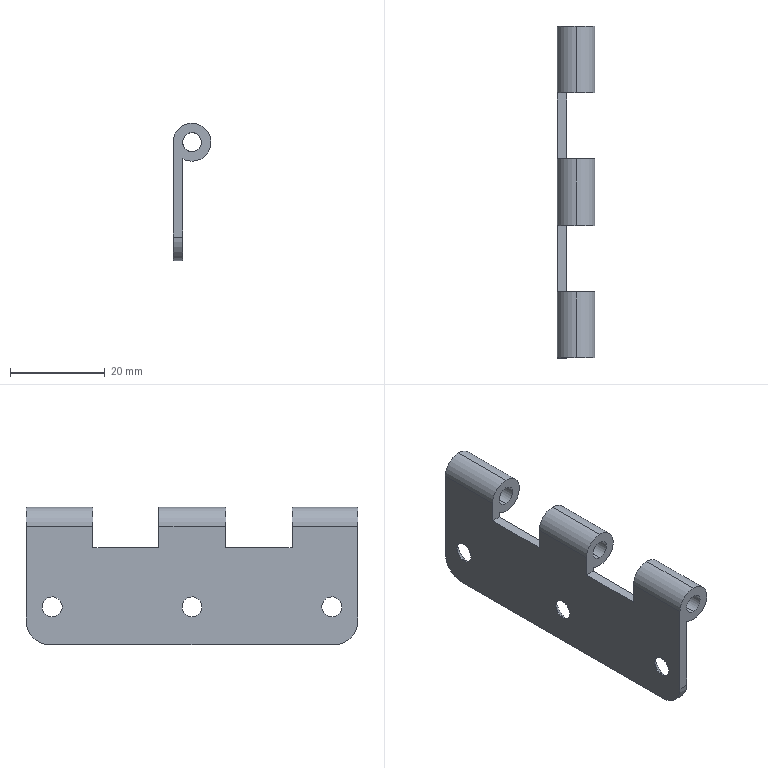Part | SolidWorks | features BaseBody 1 | 1 solid | 40 faces | box 8 x 70 x 29 mm | volume 4432 mm3 | cylinder 23 | plane 11 | cone 6 | commonest cylinder face diameters 8 x9 4 x6 4.2 x6 10 x2